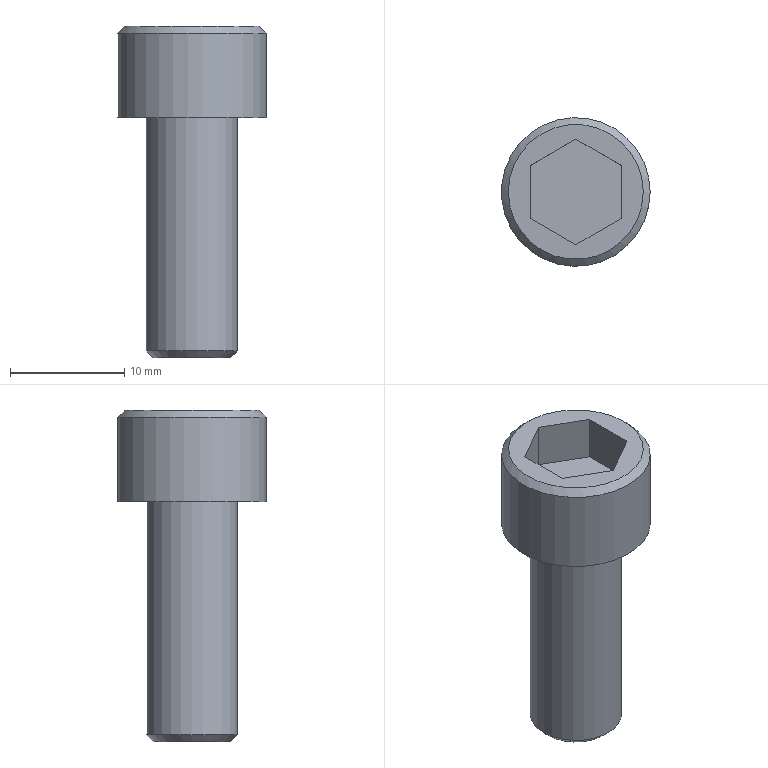Part | STEP file | solid 69 | 1 solid | 14 faces | box 13 x 13 x 29 mm | volume 1884 mm3 | plane 10 | cylinder 2 | cone 2 | commonest cylinder face diameters 8 x1 13 x1